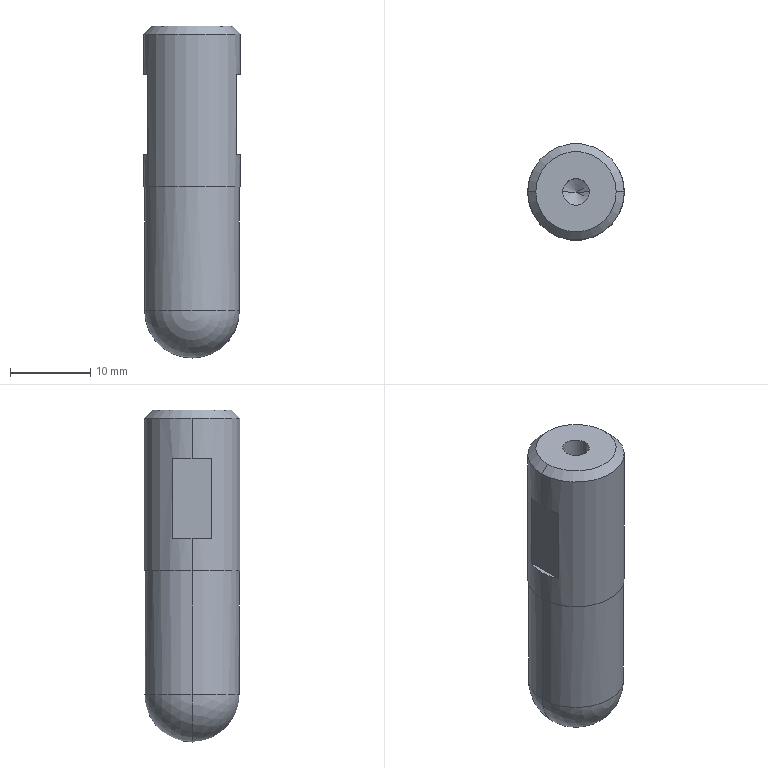Part | SolidWorks | features ICE 2, Chamfer 1, Extrusion 1, HoleWzd 1, Revolution 1 | 1 solid | 20 faces | box 12 x 12 x 41.3 mm | volume 4237 mm3 | plane 8 | cylinder 6 | cone 4 | sphere 2 | commonest cylinder face diameters 3.3 x2 11.8 x2 12 x2
STEP:
#1=CARTESIAN_POINT('',(5.,0.,35.4));
#2=VERTEX_POINT('',#1);
#3=CARTESIAN_POINT('',(-5.,0.,35.4));
#4=VERTEX_POINT('',#3);
#5=CARTESIAN_POINT('',(0.,0.,35.4));
#6=DIRECTION('',(0.,0.,1.));
#7=DIRECTION('',(1.,0.,0.));
#8=AXIS2_PLACEMENT_3D('',#5,#6,#7);
#9=CIRCLE('',#8,5.);
#10=EDGE_CURVE('',#2,#4,#9,.T.);
#11=ORIENTED_EDGE('',*,*,#10,.F.);
#12=CARTESIAN_POINT('',(6.,0.,34.4));
#13=VERTEX_POINT('',#12);
#14=CARTESIAN_POINT('',(5.,0.,35.4));
#15=DIRECTION('',(0.7071,0.,-0.7071));
#16=VECTOR('',#15,1000.);
#17=LINE('',#14,#16);
#18=EDGE_CURVE('',#2,#13,#17,.T.);
#19=ORIENTED_EDGE('',*,*,#18,.T.);
#20=CARTESIAN_POINT('',(-6.,0.,34.4));
#21=VERTEX_POINT('',#20);
#22=CARTESIAN_POINT('',(0.,0.,34.4));
#23=DIRECTION('',(0.,0.,-1.));
#24=DIRECTION('',(1.,0.,0.));
#25=AXIS2_PLACEMENT_3D('',#22,#23,#24);
#26=CIRCLE('',#25,6.);
#27=EDGE_CURVE('',#21,#13,#26,.T.);
#28=ORIENTED_EDGE('',*,*,#27,.F.);
#29=CARTESIAN_POINT('',(-5.,0.,35.4));
#30=DIRECTION('',(-0.7071,0.,-0.7071));
#31=VECTOR('',#30,1000.);
#32=LINE('',#29,#31);
#33=EDGE_CURVE('',#4,#21,#32,.T.);
#34=ORIENTED_EDGE('',*,*,#33,.F.);
#35=EDGE_LOOP('',(#11,#19,#28,#34));
#36=FACE_OUTER_BOUND('',#35,.T.);
#37=CARTESIAN_POINT('',(0.,0.,35.4));
#38=DIRECTION('',(0.,0.,-1.));
#39=DIRECTION('',(-1.,0.,0.));
#40=AXIS2_PLACEMENT_3D('',#37,#38,#39);
#41=CONICAL_SURFACE('',#40,5.,0.7854);
#42=ADVANCED_FACE('',(#36),#41,.T.);
#43=CARTESIAN_POINT('',(5.9,0.,15.4));
#44=VERTEX_POINT('',#43);
#45=CARTESIAN_POINT('',(-5.9,0.,15.4));
#46=VERTEX_POINT('',#45);
#47=CARTESIAN_POINT('',(0.,0.,15.4));
#48=DIRECTION('',(0.,0.,1.));
#49=DIRECTION('',(1.,0.,0.));
#50=AXIS2_PLACEMENT_3D('',#47,#48,#49);
#51=CIRCLE('',#50,5.9);
#52=EDGE_CURVE('',#44,#46,#51,.T.);
#53=ORIENTED_EDGE('',*,*,#52,.F.);
#54=CARTESIAN_POINT('',(5.9,0.,0.));
#55=VERTEX_POINT('',#54);
#56=CARTESIAN_POINT('',(5.9,0.,35.4));
#57=DIRECTION('',(0.,0.,-1.));
#58=VECTOR('',#57,1000.);
#59=LINE('',#56,#58);
#60=EDGE_CURVE('',#44,#55,#59,.T.);
#61=ORIENTED_EDGE('',*,*,#60,.T.);
#62=CARTESIAN_POINT('',(-5.9,0.,0.));
#63=VERTEX_POINT('',#62);
#64=CARTESIAN_POINT('',(0.,0.,0.));
#65=DIRECTION('',(0.,0.,-1.));
#66=DIRECTION('',(-1.,0.,0.));
#67=AXIS2_PLACEMENT_3D('',#64,#65,#66);
#68=CIRCLE('',#67,5.9);
#69=EDGE_CURVE('',#63,#55,#68,.T.);
#70=ORIENTED_EDGE('',*,*,#69,.F.);
#71=CARTESIAN_POINT('',(-5.9,0.,35.4));
#72=DIRECTION('',(0.,0.,-1.));
#73=VECTOR('',#72,1000.);
#74=LINE('',#71,#73);
#75=EDGE_CURVE('',#46,#63,#74,.T.);
#76=ORIENTED_EDGE('',*,*,#75,.F.);
#77=EDGE_LOOP('',(#53,#61,#70,#76));
#78=FACE_OUTER_BOUND('',#77,.T.);
#79=CARTESIAN_POINT('',(0.,0.,35.4));
#80=DIRECTION('',(0.,0.,-1.));
#81=DIRECTION('',(-1.,0.,0.));
#82=AXIS2_PLACEMENT_3D('',#79,#80,#81);
#83=CYLINDRICAL_SURFACE('',#82,5.9);
#84=ADVANCED_FACE('',(#78),#83,.T.);
#85=ORIENTED_EDGE('',*,*,#69,.T.);
#86=CARTESIAN_POINT('',(0.,0.,-5.9));
#87=VERTEX_POINT('',#86);
#88=CARTESIAN_POINT('',(0.,0.,0.));
#89=DIRECTION('',(0.,1.,0.));
#90=DIRECTION('',(-1.,0.,0.));
#91=AXIS2_PLACEMENT_3D('',#88,#89,#90);
#92=CIRCLE('',#91,5.9);
#93=EDGE_CURVE('',#55,#87,#92,.T.);
#94=ORIENTED_EDGE('',*,*,#93,.T.);
#95=CARTESIAN_POINT('',(0.,0.,0.));
#96=DIRECTION('',(0.,-1.,0.));
#97=DIRECTION('',(0.,0.,-1.));
#98=AXIS2_PLACEMENT_3D('',#95,#96,#97);
#99=CIRCLE('',#98,5.9);
#100=EDGE_CURVE('',#63,#87,#99,.T.);
#101=ORIENTED_EDGE('',*,*,#100,.F.);
#102=EDGE_LOOP('',(#85,#94,#101));
#103=FACE_OUTER_BOUND('',#102,.T.);
#104=CARTESIAN_POINT('',(0.,0.,0.));
#105=DIRECTION('',(0.,1.,0.));
#106=DIRECTION('',(-1.,0.,0.));
#107=AXIS2_PLACEMENT_3D('',#104,#105,#106);
#108=SPHERICAL_SURFACE('',#107,5.9);
#109=ADVANCED_FACE('',(#103),#108,.T.);
#110=CARTESIAN_POINT('',(6.,0.,15.4));
#111=VERTEX_POINT('',#110);
#112=CARTESIAN_POINT('',(-6.,0.,15.4));
#113=VERTEX_POINT('',#112);
#114=CARTESIAN_POINT('',(0.,0.,15.4));
#115=DIRECTION('',(0.,0.,1.));
#116=DIRECTION('',(1.,0.,0.));
#117=AXIS2_PLACEMENT_3D('',#114,#115,#116);
#118=CIRCLE('',#117,6.);
#119=EDGE_CURVE('',#111,#113,#118,.T.);
#120=ORIENTED_EDGE('',*,*,#119,.T.);
#121=CARTESIAN_POINT('',(-6.,0.,19.4));
#122=VERTEX_POINT('',#121);
#123=CARTESIAN_POINT('',(-6.,0.,15.4));
#124=DIRECTION('',(0.,0.,1.));
#125=VECTOR('',#124,1000.);
#126=LINE('',#123,#125);
#127=EDGE_CURVE('',#113,#122,#126,.T.);
#128=ORIENTED_EDGE('',*,*,#127,.T.);
#129=CARTESIAN_POINT('',(-5.5,2.398,19.4));
#130=VERTEX_POINT('',#129);
#131=CARTESIAN_POINT('',(0.,0.,19.4));
#132=DIRECTION('',(0.,0.,1.));
#133=DIRECTION('',(-1.,0.,0.));
#134=AXIS2_PLACEMENT_3D('',#131,#132,#133);
#135=CIRCLE('',#134,6.);
#136=EDGE_CURVE('',#130,#122,#135,.T.);
#137=ORIENTED_EDGE('',*,*,#136,.F.);
#138=CARTESIAN_POINT('',(-5.5,2.398,29.4));
#139=VERTEX_POINT('',#138);
#140=CARTESIAN_POINT('',(-5.5,2.398,15.4));
#141=DIRECTION('',(0.,0.,-1.));
#142=VECTOR('',#141,1000.);
#143=LINE('',#140,#142);
#144=EDGE_CURVE('',#139,#130,#143,.T.);
#145=ORIENTED_EDGE('',*,*,#144,.F.);
#146=CARTESIAN_POINT('',(-6.,0.,29.4));
#147=VERTEX_POINT('',#146);
#148=CARTESIAN_POINT('',(0.,0.,29.4));
#149=DIRECTION('',(0.,0.,-1.));
#150=DIRECTION('',(1.,0.,0.));
#151=AXIS2_PLACEMENT_3D('',#148,#149,#150);
#152=CIRCLE('',#151,6.);
#153=EDGE_CURVE('',#147,#139,#152,.T.);
#154=ORIENTED_EDGE('',*,*,#153,.F.);
#155=CARTESIAN_POINT('',(-6.,0.,15.4));
#156=DIRECTION('',(0.,0.,1.));
#157=VECTOR('',#156,1000.);
#158=LINE('',#155,#157);
#159=EDGE_CURVE('',#147,#21,#158,.T.);
#160=ORIENTED_EDGE('',*,*,#159,.T.);
#161=ORIENTED_EDGE('',*,*,#27,.T.);
#162=CARTESIAN_POINT('',(6.,0.,29.4));
#163=VERTEX_POINT('',#162);
#164=CARTESIAN_POINT('',(6.,0.,15.4));
#165=DIRECTION('',(0.,0.,1.));
#166=VECTOR('',#165,1000.);
#167=LINE('',#164,#166);
#168=EDGE_CURVE('',#163,#13,#167,.T.);
#169=ORIENTED_EDGE('',*,*,#168,.F.);
#170=CARTESIAN_POINT('',(5.5,2.398,29.4));
#171=VERTEX_POINT('',#170);
#172=CARTESIAN_POINT('',(0.,0.,29.4));
#173=DIRECTION('',(0.,0.,-1.));
#174=DIRECTION('',(1.,0.,0.));
#175=AXIS2_PLACEMENT_3D('',#172,#173,#174);
#176=CIRCLE('',#175,6.);
#177=EDGE_CURVE('',#171,#163,#176,.T.);
#178=ORIENTED_EDGE('',*,*,#177,.F.);
#179=CARTESIAN_POINT('',(5.5,2.398,19.4));
#180=VERTEX_POINT('',#179);
#181=CARTESIAN_POINT('',(5.5,2.398,15.4));
#182=DIRECTION('',(0.,0.,1.));
#183=VECTOR('',#182,1000.);
#184=LINE('',#181,#183);
#185=EDGE_CURVE('',#180,#171,#184,.T.);
#186=ORIENTED_EDGE('',*,*,#185,.F.);
#187=CARTESIAN_POINT('',(6.,0.,19.4));
#188=VERTEX_POINT('',#187);
#189=CARTESIAN_POINT('',(0.,0.,19.4));
#190=DIRECTION('',(0.,0.,1.));
#191=DIRECTION('',(-1.,0.,0.));
#192=AXIS2_PLACEMENT_3D('',#189,#190,#191);
#193=CIRCLE('',#192,6.);
#194=EDGE_CURVE('',#188,#180,#193,.T.);
#195=ORIENTED_EDGE('',*,*,#194,.F.);
#196=CARTESIAN_POINT('',(6.,0.,15.4));
#197=DIRECTION('',(0.,0.,1.));
#198=VECTOR('',#197,1000.);
#199=LINE('',#196,#198);
#200=EDGE_CURVE('',#111,#188,#199,.T.);
#201=ORIENTED_EDGE('',*,*,#200,.F.);
#202=EDGE_LOOP('',(#120,#128,#137,#145,#154,#160,#161,#169,#178,#186,#195,#201));
#203=FACE_OUTER_BOUND('',#202,.T.);
#204=CARTESIAN_POINT('',(0.,0.,15.4));
#205=DIRECTION('',(0.,0.,1.));
#206=DIRECTION('',(1.,0.,0.));
#207=AXIS2_PLACEMENT_3D('',#204,#205,#206);
#208=CYLINDRICAL_SURFACE('',#207,6.);
#209=ADVANCED_FACE('',(#203),#208,.T.);
#210=CARTESIAN_POINT('',(-1.65,0.,25.3));
#211=VERTEX_POINT('',#210);
#212=CARTESIAN_POINT('',(1.65,0.,25.3));
#213=VERTEX_POINT('',#212);
#214=CARTESIAN_POINT('',(0.,0.,25.3));
#215=DIRECTION('',(0.,0.,1.));
#216=DIRECTION('',(1.,0.,0.));
#217=AXIS2_PLACEMENT_3D('',#214,#215,#216);
#218=CIRCLE('',#217,1.65);
#219=EDGE_CURVE('',#211,#213,#218,.T.);
#220=ORIENTED_EDGE('',*,*,#219,.F.);
#221=CARTESIAN_POINT('',(-1.65,0.,35.4));
#222=VERTEX_POINT('',#221);
#223=CARTESIAN_POINT('',(-1.65,0.,35.4));
#224=DIRECTION('',(0.,0.,1.));
#225=VECTOR('',#224,1000.);
#226=LINE('',#223,#225);
#227=EDGE_CURVE('',#211,#222,#226,.T.);
#228=ORIENTED_EDGE('',*,*,#227,.T.);
#229=CARTESIAN_POINT('',(1.65,0.,35.4));
#230=VERTEX_POINT('',#229);
#231=CARTESIAN_POINT('',(0.,0.,35.4));
#232=DIRECTION('',(0.,0.,1.));
#233=DIRECTION('',(1.,0.,0.));
#234=AXIS2_PLACEMENT_3D('',#231,#232,#233);
#235=CIRCLE('',#234,1.65);
#236=EDGE_CURVE('',#222,#230,#235,.T.);
#237=ORIENTED_EDGE('',*,*,#236,.T.);
#238=CARTESIAN_POINT('',(1.65,0.,35.4));
#239=DIRECTION('',(0.,0.,1.));
#240=VECTOR('',#239,1000.);
#241=LINE('',#238,#240);
#242=EDGE_CURVE('',#213,#230,#241,.T.);
#243=ORIENTED_EDGE('',*,*,#242,.F.);
#244=EDGE_LOOP('',(#220,#228,#237,#243));
#245=FACE_OUTER_BOUND('',#244,.T.);
#246=CARTESIAN_POINT('',(0.,0.,35.4));
#247=DIRECTION('',(0.,0.,1.));
#248=DIRECTION('',(1.,0.,0.));
#249=AXIS2_PLACEMENT_3D('',#246,#247,#248);
#250=CYLINDRICAL_SURFACE('',#249,1.65);
#251=ADVANCED_FACE('',(#245),#250,.F.);
#252=CARTESIAN_POINT('',(0.,0.,24.309));
#253=VERTEX_POINT('',#252);
#254=CARTESIAN_POINT('',(1.65,0.,25.3));
#255=DIRECTION('',(0.8572,0.,0.515));
#256=VECTOR('',#255,1000.);
#257=LINE('',#254,#256);
#258=EDGE_CURVE('',#253,#213,#257,.T.);
#259=ORIENTED_EDGE('',*,*,#258,.F.);
#260=CARTESIAN_POINT('',(-1.65,0.,25.3));
#261=DIRECTION('',(-0.8572,0.,0.515));
#262=VECTOR('',#261,1000.);
#263=LINE('',#260,#262);
#264=EDGE_CURVE('',#253,#211,#263,.T.);
#265=ORIENTED_EDGE('',*,*,#264,.T.);
#266=ORIENTED_EDGE('',*,*,#219,.T.);
#267=EDGE_LOOP('',(#259,#265,#266));
#268=FACE_OUTER_BOUND('',#267,.T.);
#269=CARTESIAN_POINT('',(0.,0.,25.3));
#270=DIRECTION('',(0.,0.,1.));
#271=DIRECTION('',(1.,0.,0.));
#272=AXIS2_PLACEMENT_3D('',#269,#270,#271);
#273=CONICAL_SURFACE('',#272,1.65,1.03);
#274=ADVANCED_FACE('',(#268),#273,.F.);
#275=CARTESIAN_POINT('',(0.,0.,35.4));
#276=DIRECTION('',(0.,0.,1.));
#277=DIRECTION('',(1.,0.,0.));
#278=AXIS2_PLACEMENT_3D('',#275,#276,#277);
#279=CIRCLE('',#278,5.);
#280=EDGE_CURVE('',#4,#2,#279,.T.);
#281=ORIENTED_EDGE('',*,*,#280,.T.);
#282=ORIENTED_EDGE('',*,*,#10,.T.);
#283=EDGE_LOOP('',(#281,#282));
#284=FACE_OUTER_BOUND('',#283,.T.);
#285=CARTESIAN_POINT('',(0.,0.,35.4));
#286=DIRECTION('',(0.,0.,1.));
#287=DIRECTION('',(1.,0.,0.));
#288=AXIS2_PLACEMENT_3D('',#285,#286,#287);
#289=CIRCLE('',#288,1.65);
#290=EDGE_CURVE('',#230,#222,#289,.T.);
#291=ORIENTED_EDGE('',*,*,#290,.F.);
#292=ORIENTED_EDGE('',*,*,#236,.F.);
#293=EDGE_LOOP('',(#291,#292));
#294=FACE_BOUND('',#293,.T.);
#295=CARTESIAN_POINT('',(0.,0.,35.4));
#296=DIRECTION('',(0.,0.,1.));
#297=DIRECTION('',(1.,0.,0.));
#298=AXIS2_PLACEMENT_3D('',#295,#296,#297);
#299=PLANE('',#298);
#300=ADVANCED_FACE('',(#284,#294),#299,.T.);
#301=ORIENTED_EDGE('',*,*,#264,.F.);
#302=ORIENTED_EDGE('',*,*,#258,.T.);
#303=CARTESIAN_POINT('',(0.,0.,25.3));
#304=DIRECTION('',(0.,0.,1.));
#305=DIRECTION('',(1.,0.,0.));
#306=AXIS2_PLACEMENT_3D('',#303,#304,#305);
#307=CIRCLE('',#306,1.65);
#308=EDGE_CURVE('',#213,#211,#307,.T.);
#309=ORIENTED_EDGE('',*,*,#308,.T.);
#310=EDGE_LOOP('',(#301,#302,#309));
#311=FACE_OUTER_BOUND('',#310,.T.);
#312=CARTESIAN_POINT('',(0.,0.,25.3));
#313=DIRECTION('',(0.,0.,1.));
#314=DIRECTION('',(1.,0.,0.));
#315=AXIS2_PLACEMENT_3D('',#312,#313,#314);
#316=CONICAL_SURFACE('',#315,1.65,1.03);
#317=ADVANCED_FACE('',(#311),#316,.F.);
#318=ORIENTED_EDGE('',*,*,#227,.F.);
#319=ORIENTED_EDGE('',*,*,#308,.F.);
#320=ORIENTED_EDGE('',*,*,#242,.T.);
#321=ORIENTED_EDGE('',*,*,#290,.T.);
#322=EDGE_LOOP('',(#318,#319,#320,#321));
#323=FACE_OUTER_BOUND('',#322,.T.);
#324=CARTESIAN_POINT('',(0.,0.,35.4));
#325=DIRECTION('',(0.,0.,1.));
#326=DIRECTION('',(1.,0.,0.));
#327=AXIS2_PLACEMENT_3D('',#324,#325,#326);
#328=CYLINDRICAL_SURFACE('',#327,1.65);
#329=ADVANCED_FACE('',(#323),#328,.F.);
#330=ORIENTED_EDGE('',*,*,#127,.F.);
#331=CARTESIAN_POINT('',(0.,0.,15.4));
#332=DIRECTION('',(0.,0.,1.));
#333=DIRECTION('',(1.,0.,0.));
#334=AXIS2_PLACEMENT_3D('',#331,#332,#333);
#335=CIRCLE('',#334,6.);
#336=EDGE_CURVE('',#113,#111,#335,.T.);
#337=ORIENTED_EDGE('',*,*,#336,.T.);
#338=ORIENTED_EDGE('',*,*,#200,.T.);
#339=CARTESIAN_POINT('',(5.5,-2.398,19.4));
#340=VERTEX_POINT('',#339);
#341=CARTESIAN_POINT('',(0.,0.,19.4));
#342=DIRECTION('',(0.,0.,1.));
#343=DIRECTION('',(-1.,0.,0.));
#344=AXIS2_PLACEMENT_3D('',#341,#342,#343);
#345=CIRCLE('',#344,6.);
#346=EDGE_CURVE('',#340,#188,#345,.T.);
#347=ORIENTED_EDGE('',*,*,#346,.F.);
#348=CARTESIAN_POINT('',(5.5,-2.398,29.4));
#349=VERTEX_POINT('',#348);
#350=CARTESIAN_POINT('',(5.5,-2.398,15.4));
#351=DIRECTION('',(0.,0.,-1.));
#352=VECTOR('',#351,1000.);
#353=LINE('',#350,#352);
#354=EDGE_CURVE('',#349,#340,#353,.T.);
#355=ORIENTED_EDGE('',*,*,#354,.F.);
#356=CARTESIAN_POINT('',(0.,0.,29.4));
#357=DIRECTION('',(0.,0.,-1.));
#358=DIRECTION('',(1.,0.,0.));
#359=AXIS2_PLACEMENT_3D('',#356,#357,#358);
#360=CIRCLE('',#359,6.);
#361=EDGE_CURVE('',#163,#349,#360,.T.);
#362=ORIENTED_EDGE('',*,*,#361,.F.);
#363=ORIENTED_EDGE('',*,*,#168,.T.);
#364=CARTESIAN_POINT('',(0.,0.,34.4));
#365=DIRECTION('',(0.,0.,-1.));
#366=DIRECTION('',(1.,0.,0.));
#367=AXIS2_PLACEMENT_3D('',#364,#365,#366);
#368=CIRCLE('',#367,6.);
#369=EDGE_CURVE('',#13,#21,#368,.T.);
#370=ORIENTED_EDGE('',*,*,#369,.T.);
#371=ORIENTED_EDGE('',*,*,#159,.F.);
#372=CARTESIAN_POINT('',(-5.5,-2.398,29.4));
#373=VERTEX_POINT('',#372);
#374=CARTESIAN_POINT('',(0.,0.,29.4));
#375=DIRECTION('',(0.,0.,-1.));
#376=DIRECTION('',(1.,0.,0.));
#377=AXIS2_PLACEMENT_3D('',#374,#375,#376);
#378=CIRCLE('',#377,6.);
#379=EDGE_CURVE('',#373,#147,#378,.T.);
#380=ORIENTED_EDGE('',*,*,#379,.F.);
#381=CARTESIAN_POINT('',(-5.5,-2.398,19.4));
#382=VERTEX_POINT('',#381);
#383=CARTESIAN_POINT('',(-5.5,-2.398,15.4));
#384=DIRECTION('',(0.,0.,1.));
#385=VECTOR('',#384,1000.);
#386=LINE('',#383,#385);
#387=EDGE_CURVE('',#382,#373,#386,.T.);
#388=ORIENTED_EDGE('',*,*,#387,.F.);
#389=CARTESIAN_POINT('',(0.,0.,19.4));
#390=DIRECTION('',(0.,0.,1.));
#391=DIRECTION('',(-1.,0.,0.));
#392=AXIS2_PLACEMENT_3D('',#389,#390,#391);
#393=CIRCLE('',#392,6.);
#394=EDGE_CURVE('',#122,#382,#393,.T.);
#395=ORIENTED_EDGE('',*,*,#394,.F.);
#396=EDGE_LOOP('',(#330,#337,#338,#347,#355,#362,#363,#370,#371,#380,#388,#395));
#397=FACE_OUTER_BOUND('',#396,.T.);
#398=CARTESIAN_POINT('',(0.,0.,15.4));
#399=DIRECTION('',(0.,0.,1.));
#400=DIRECTION('',(1.,0.,0.));
#401=AXIS2_PLACEMENT_3D('',#398,#399,#400);
#402=CYLINDRICAL_SURFACE('',#401,6.);
#403=ADVANCED_FACE('',(#397),#402,.T.);
#404=CARTESIAN_POINT('',(0.,0.,15.4));
#405=DIRECTION('',(0.,0.,1.));
#406=DIRECTION('',(1.,0.,0.));
#407=AXIS2_PLACEMENT_3D('',#404,#405,#406);
#408=CIRCLE('',#407,5.9);
#409=EDGE_CURVE('',#46,#44,#408,.T.);
#410=ORIENTED_EDGE('',*,*,#409,.T.);
#411=ORIENTED_EDGE('',*,*,#52,.T.);
#412=EDGE_LOOP('',(#410,#411));
#413=FACE_BOUND('',#412,.T.);
#414=ORIENTED_EDGE('',*,*,#119,.F.);
#415=ORIENTED_EDGE('',*,*,#336,.F.);
#416=EDGE_LOOP('',(#414,#415));
#417=FACE_OUTER_BOUND('',#416,.T.);
#418=CARTESIAN_POINT('',(0.,0.,15.4));
#419=DIRECTION('',(0.,0.,1.));
#420=DIRECTION('',(1.,0.,0.));
#421=AXIS2_PLACEMENT_3D('',#418,#419,#420);
#422=PLANE('',#421);
#423=ADVANCED_FACE('',(#413,#417),#422,.F.);
#424=ORIENTED_EDGE('',*,*,#93,.F.);
#425=CARTESIAN_POINT('',(0.,0.,0.));
#426=DIRECTION('',(0.,0.,-1.));
#427=DIRECTION('',(-1.,0.,0.));
#428=AXIS2_PLACEMENT_3D('',#425,#426,#427);
#429=CIRCLE('',#428,5.9);
#430=EDGE_CURVE('',#55,#63,#429,.T.);
#431=ORIENTED_EDGE('',*,*,#430,.T.);
#432=ORIENTED_EDGE('',*,*,#100,.T.);
#433=EDGE_LOOP('',(#424,#431,#432));
#434=FACE_OUTER_BOUND('',#433,.T.);
#435=CARTESIAN_POINT('',(0.,0.,0.));
#436=DIRECTION('',(0.,1.,0.));
#437=DIRECTION('',(-1.,0.,0.));
#438=AXIS2_PLACEMENT_3D('',#435,#436,#437);
#439=SPHERICAL_SURFACE('',#438,5.9);
#440=ADVANCED_FACE('',(#434),#439,.T.);
#441=ORIENTED_EDGE('',*,*,#60,.F.);
#442=ORIENTED_EDGE('',*,*,#409,.F.);
#443=ORIENTED_EDGE('',*,*,#75,.T.);
#444=ORIENTED_EDGE('',*,*,#430,.F.);
#445=EDGE_LOOP('',(#441,#442,#443,#444));
#446=FACE_OUTER_BOUND('',#445,.T.);
#447=CARTESIAN_POINT('',(0.,0.,35.4));
#448=DIRECTION('',(0.,0.,-1.));
#449=DIRECTION('',(-1.,0.,0.));
#450=AXIS2_PLACEMENT_3D('',#447,#448,#449);
#451=CYLINDRICAL_SURFACE('',#450,5.9);
#452=ADVANCED_FACE('',(#446),#451,.T.);
#453=ORIENTED_EDGE('',*,*,#18,.F.);
#454=ORIENTED_EDGE('',*,*,#280,.F.);
#455=ORIENTED_EDGE('',*,*,#33,.T.);
#456=ORIENTED_EDGE('',*,*,#369,.F.);
#457=EDGE_LOOP('',(#453,#454,#455,#456));
#458=FACE_OUTER_BOUND('',#457,.T.);
#459=CARTESIAN_POINT('',(0.,0.,35.4));
#460=DIRECTION('',(0.,0.,-1.));
#461=DIRECTION('',(-1.,0.,0.));
#462=AXIS2_PLACEMENT_3D('',#459,#460,#461);
#463=CONICAL_SURFACE('',#462,5.,0.7854);
#464=ADVANCED_FACE('',(#458),#463,.T.);
#465=ORIENTED_EDGE('',*,*,#177,.T.);
#466=ORIENTED_EDGE('',*,*,#361,.T.);
#467=CARTESIAN_POINT('',(5.5,-6.,29.4));
#468=DIRECTION('',(0.,1.,0.));
#469=VECTOR('',#468,1000.);
#470=LINE('',#467,#469);
#471=EDGE_CURVE('',#349,#171,#470,.T.);
#472=ORIENTED_EDGE('',*,*,#471,.T.);
#473=EDGE_LOOP('',(#465,#466,#472));
#474=FACE_OUTER_BOUND('',#473,.T.);
#475=CARTESIAN_POINT('',(7.526,-6.,29.4));
#476=DIRECTION('',(0.,0.,1.));
#477=DIRECTION('',(1.,0.,0.));
#478=AXIS2_PLACEMENT_3D('',#475,#476,#477);
#479=PLANE('',#478);
#480=ADVANCED_FACE('',(#474),#479,.F.);
#481=ORIENTED_EDGE('',*,*,#354,.T.);
#482=CARTESIAN_POINT('',(5.5,-6.,19.4));
#483=DIRECTION('',(0.,1.,0.));
#484=VECTOR('',#483,1000.);
#485=LINE('',#482,#484);
#486=EDGE_CURVE('',#340,#180,#485,.T.);
#487=ORIENTED_EDGE('',*,*,#486,.T.);
#488=ORIENTED_EDGE('',*,*,#185,.T.);
#489=ORIENTED_EDGE('',*,*,#471,.F.);
#490=EDGE_LOOP('',(#481,#487,#488,#489));
#491=FACE_OUTER_BOUND('',#490,.T.);
#492=CARTESIAN_POINT('',(5.5,-6.,19.4));
#493=DIRECTION('',(-1.,0.,0.));
#494=DIRECTION('',(0.,0.,1.));
#495=AXIS2_PLACEMENT_3D('',#492,#493,#494);
#496=PLANE('',#495);
#497=ADVANCED_FACE('',(#491),#496,.F.);
#498=ORIENTED_EDGE('',*,*,#346,.T.);
#499=ORIENTED_EDGE('',*,*,#194,.T.);
#500=ORIENTED_EDGE('',*,*,#486,.F.);
#501=EDGE_LOOP('',(#498,#499,#500));
#502=FACE_OUTER_BOUND('',#501,.T.);
#503=CARTESIAN_POINT('',(7.526,-6.,19.4));
#504=DIRECTION('',(0.,0.,-1.));
#505=DIRECTION('',(-1.,0.,0.));
#506=AXIS2_PLACEMENT_3D('',#503,#504,#505);
#507=PLANE('',#506);
#508=ADVANCED_FACE('',(#502),#507,.F.);
#509=ORIENTED_EDGE('',*,*,#136,.T.);
#510=ORIENTED_EDGE('',*,*,#394,.T.);
#511=CARTESIAN_POINT('',(-5.5,-6.,19.4));
#512=DIRECTION('',(0.,1.,0.));
#513=VECTOR('',#512,1000.);
#514=LINE('',#511,#513);
#515=EDGE_CURVE('',#382,#130,#514,.T.);
#516=ORIENTED_EDGE('',*,*,#515,.T.);
#517=EDGE_LOOP('',(#509,#510,#516));
#518=FACE_OUTER_BOUND('',#517,.T.);
#519=CARTESIAN_POINT('',(-7.526,-6.,19.4));
#520=DIRECTION('',(0.,0.,-1.));
#521=DIRECTION('',(-1.,0.,0.));
#522=AXIS2_PLACEMENT_3D('',#519,#520,#521);
#523=PLANE('',#522);
#524=ADVANCED_FACE('',(#518),#523,.F.);
#525=ORIENTED_EDGE('',*,*,#144,.T.);
#526=ORIENTED_EDGE('',*,*,#515,.F.);
#527=ORIENTED_EDGE('',*,*,#387,.T.);
#528=CARTESIAN_POINT('',(-5.5,-6.,29.4));
#529=DIRECTION('',(0.,1.,0.));
#530=VECTOR('',#529,1000.);
#531=LINE('',#528,#530);
#532=EDGE_CURVE('',#373,#139,#531,.T.);
#533=ORIENTED_EDGE('',*,*,#532,.T.);
#534=EDGE_LOOP('',(#525,#526,#527,#533));
#535=FACE_OUTER_BOUND('',#534,.T.);
#536=CARTESIAN_POINT('',(-5.5,-6.,19.4));
#537=DIRECTION('',(1.,0.,0.));
#538=DIRECTION('',(0.,0.,-1.));
#539=AXIS2_PLACEMENT_3D('',#536,#537,#538);
#540=PLANE('',#539);
#541=ADVANCED_FACE('',(#535),#540,.F.);
#542=ORIENTED_EDGE('',*,*,#379,.T.);
#543=ORIENTED_EDGE('',*,*,#153,.T.);
#544=ORIENTED_EDGE('',*,*,#532,.F.);
#545=EDGE_LOOP('',(#542,#543,#544));
#546=FACE_OUTER_BOUND('',#545,.T.);
#547=CARTESIAN_POINT('',(-7.526,-6.,29.4));
#548=DIRECTION('',(0.,0.,1.));
#549=DIRECTION('',(1.,0.,0.));
#550=AXIS2_PLACEMENT_3D('',#547,#548,#549);
#551=PLANE('',#550);
#552=ADVANCED_FACE('',(#546),#551,.F.);
#553=CLOSED_SHELL('',(#42,#84,#109,#209,#251,#274,#300,#317,#329,#403,#423,#440,#452,#464,#480,#497,#508,#524,#541,#552));
#554=MANIFOLD_SOLID_BREP('',#553);
#555=CARTESIAN_POINT('',(0.,0.,0.));
#556=DIRECTION('',(0.,0.,1.));
#557=DIRECTION('',(1.,0.,0.));
#558=AXIS2_PLACEMENT_3D('',#555,#556,#557);
#559=(LENGTH_UNIT()NAMED_UNIT(*)SI_UNIT(.MILLI.,.METRE.));
#560=UNCERTAINTY_MEASURE_WITH_UNIT(LENGTH_MEASURE(0.00001),#559,'','');
#561=(NAMED_UNIT(*)PLANE_ANGLE_UNIT()SI_UNIT($,.RADIAN.));
#562=(NAMED_UNIT(*)SI_UNIT($,.STERADIAN.)SOLID_ANGLE_UNIT());
#563=(GEOMETRIC_REPRESENTATION_CONTEXT(3)GLOBAL_UNCERTAINTY_ASSIGNED_CONTEXT((#560))GLOBAL_UNIT_ASSIGNED_CONTEXT((#559,#561,#562))REPRESENTATION_CONTEXT('',''));
#564=ADVANCED_BREP_SHAPE_REPRESENTATION('',(#554,#558),#563);